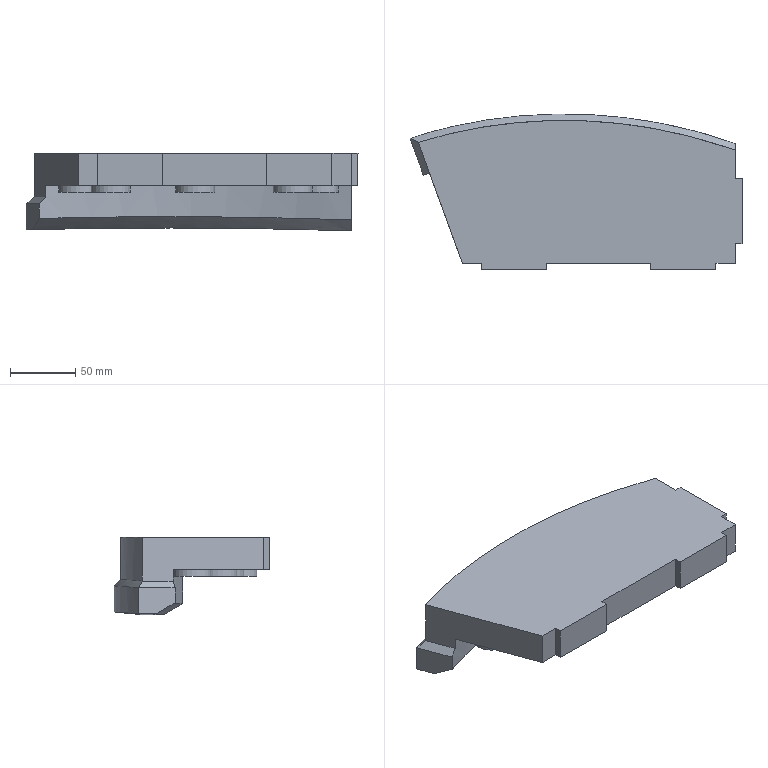Part | NX | features solid 2 | 1 solid | 35 faces | box 254.998 x 119.823 x 59.692 mm | volume 840933 mm3 | plane 24 | spline 6 | cylinder 5 | commonest cylinder face diameters 30 x5